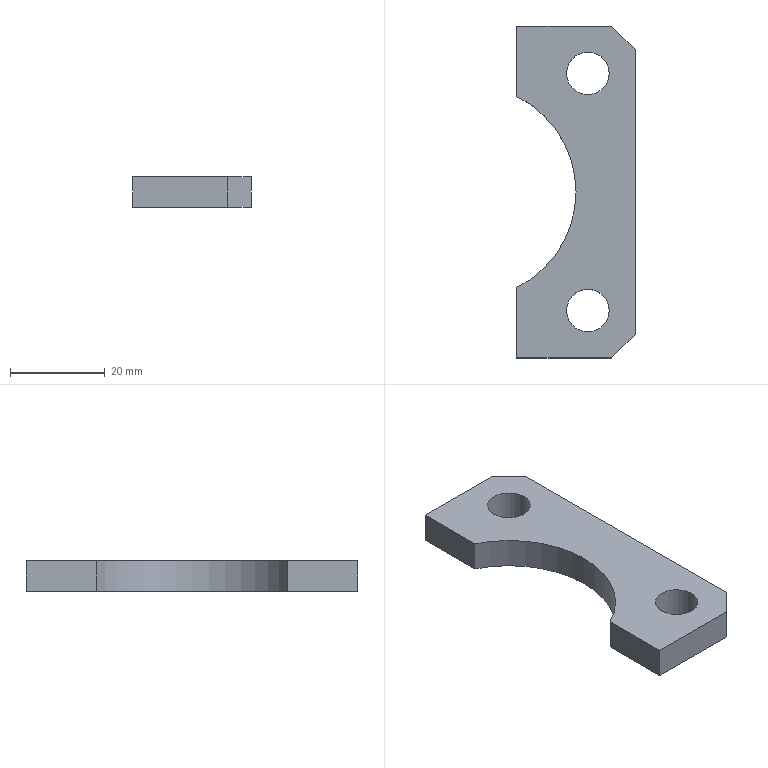Part | NX | features solid 2 | 1 solid | 12 faces | box 25 x 70 x 6.5 mm | volume 8042 mm3 | plane 9 | cylinder 3 | commonest cylinder face diameters 9 x2 45 x1
STEP:
#1=CARTESIAN_POINT('',(-840.,-430.,-48.49));
#2=VERTEX_POINT('',#1);
#3=CARTESIAN_POINT('',(-840.,-490.,-48.49));
#4=VERTEX_POINT('',#3);
#5=CARTESIAN_POINT('',(-840.,-325.,-48.49));
#6=DIRECTION('',(0.,1.,0.));
#7=VECTOR('',#6,1000.);
#8=LINE('',#5,#7);
#9=EDGE_CURVE('',#2,#4,#8,.F.);
#10=ORIENTED_EDGE('',*,*,#9,.T.);
#11=CARTESIAN_POINT('',(-840.,-490.,-54.99));
#12=VERTEX_POINT('',#11);
#13=CARTESIAN_POINT('',(-840.,-490.,-54.99));
#14=DIRECTION('',(0.,0.,-1.));
#15=VECTOR('',#14,1000.);
#16=LINE('',#13,#15);
#17=EDGE_CURVE('',#4,#12,#16,.T.);
#18=ORIENTED_EDGE('',*,*,#17,.T.);
#19=CARTESIAN_POINT('',(-840.,-430.,-54.99));
#20=VERTEX_POINT('',#19);
#21=CARTESIAN_POINT('',(-840.,-325.,-54.99));
#22=DIRECTION('',(0.,1.,0.));
#23=VECTOR('',#22,1000.);
#24=LINE('',#21,#23);
#25=EDGE_CURVE('',#20,#12,#24,.F.);
#26=ORIENTED_EDGE('',*,*,#25,.F.);
#27=CARTESIAN_POINT('',(-840.,-430.,-48.49));
#28=DIRECTION('',(0.,0.,1.));
#29=VECTOR('',#28,1000.);
#30=LINE('',#27,#29);
#31=EDGE_CURVE('',#20,#2,#30,.T.);
#32=ORIENTED_EDGE('',*,*,#31,.T.);
#33=EDGE_LOOP('',(#10,#18,#26,#32));
#34=FACE_BOUND('',#33,.T.);
#35=CARTESIAN_POINT('',(-840.,-325.,-54.99));
#36=DIRECTION('',(-1.,0.,0.));
#37=DIRECTION('',(0.,0.,-1.));
#38=AXIS2_PLACEMENT_3D('',#35,#36,#37);
#39=PLANE('',#38);
#40=ADVANCED_FACE('',(#34),#39,.F.);
#41=CARTESIAN_POINT('',(-865.,-439.844,-48.49));
#42=VERTEX_POINT('',#41);
#43=CARTESIAN_POINT('',(-865.,-439.844,-54.99));
#44=VERTEX_POINT('',#43);
#45=CARTESIAN_POINT('',(-865.,-439.844,-54.99));
#46=DIRECTION('',(0.,0.,1.));
#47=VECTOR('',#46,1000.);
#48=LINE('',#45,#47);
#49=EDGE_CURVE('',#42,#44,#48,.F.);
#50=ORIENTED_EDGE('',*,*,#49,.T.);
#51=CARTESIAN_POINT('',(-865.,-480.156,-54.99));
#52=VERTEX_POINT('',#51);
#53=CARTESIAN_POINT('',(-875.,-460.,-54.99));
#54=DIRECTION('',(0.,0.,1.));
#55=DIRECTION('',(-1.,0.,0.));
#56=AXIS2_PLACEMENT_3D('',#53,#54,#55);
#57=CIRCLE('',#56,22.5);
#58=EDGE_CURVE('',#52,#44,#57,.T.);
#59=ORIENTED_EDGE('',*,*,#58,.F.);
#60=CARTESIAN_POINT('',(-865.,-480.156,-48.49));
#61=VERTEX_POINT('',#60);
#62=CARTESIAN_POINT('',(-865.,-480.156,-54.99));
#63=DIRECTION('',(0.,0.,1.));
#64=VECTOR('',#63,1000.);
#65=LINE('',#62,#64);
#66=EDGE_CURVE('',#52,#61,#65,.T.);
#67=ORIENTED_EDGE('',*,*,#66,.T.);
#68=CARTESIAN_POINT('',(-875.,-460.,-48.49));
#69=DIRECTION('',(0.,0.,1.));
#70=DIRECTION('',(-1.,0.,0.));
#71=AXIS2_PLACEMENT_3D('',#68,#69,#70);
#72=CIRCLE('',#71,22.5);
#73=EDGE_CURVE('',#42,#61,#72,.F.);
#74=ORIENTED_EDGE('',*,*,#73,.F.);
#75=EDGE_LOOP('',(#50,#59,#67,#74));
#76=FACE_BOUND('',#75,.T.);
#77=CARTESIAN_POINT('',(-875.,-460.,-54.99));
#78=DIRECTION('',(0.,0.,1.));
#79=DIRECTION('',(-1.,0.,0.));
#80=AXIS2_PLACEMENT_3D('',#77,#78,#79);
#81=CYLINDRICAL_SURFACE('',#80,22.5);
#82=ADVANCED_FACE('',(#76),#81,.F.);
#83=CARTESIAN_POINT('',(-845.5,-485.,-48.49));
#84=VERTEX_POINT('',#83);
#85=CARTESIAN_POINT('',(-850.,-485.,-48.49));
#86=DIRECTION('',(0.,0.,-1.));
#87=DIRECTION('',(1.,0.,0.));
#88=AXIS2_PLACEMENT_3D('',#85,#86,#87);
#89=CIRCLE('',#88,4.5);
#90=EDGE_CURVE('',#84,#84,#89,.T.);
#91=ORIENTED_EDGE('',*,*,#90,.T.);
#92=EDGE_LOOP('',(#91));
#93=FACE_BOUND('',#92,.T.);
#94=CARTESIAN_POINT('',(-845.5,-435.,-48.49));
#95=VERTEX_POINT('',#94);
#96=CARTESIAN_POINT('',(-850.,-435.,-48.49));
#97=DIRECTION('',(0.,0.,-1.));
#98=DIRECTION('',(1.,0.,0.));
#99=AXIS2_PLACEMENT_3D('',#96,#97,#98);
#100=CIRCLE('',#99,4.5);
#101=EDGE_CURVE('',#95,#95,#100,.T.);
#102=ORIENTED_EDGE('',*,*,#101,.T.);
#103=EDGE_LOOP('',(#102));
#104=FACE_BOUND('',#103,.T.);
#105=CARTESIAN_POINT('',(-845.,-495.,-48.49));
#106=VERTEX_POINT('',#105);
#107=CARTESIAN_POINT('',(-865.,-495.,-48.49));
#108=VERTEX_POINT('',#107);
#109=CARTESIAN_POINT('',(-1090.,-495.,-48.49));
#110=DIRECTION('',(1.,0.,0.));
#111=VECTOR('',#110,1000.);
#112=LINE('',#109,#111);
#113=EDGE_CURVE('',#106,#108,#112,.F.);
#114=ORIENTED_EDGE('',*,*,#113,.F.);
#115=CARTESIAN_POINT('',(-845.,-495.,-48.49));
#116=DIRECTION('',(0.7071,0.7071,0.));
#117=VECTOR('',#116,1000.);
#118=LINE('',#115,#117);
#119=EDGE_CURVE('',#106,#4,#118,.T.);
#120=ORIENTED_EDGE('',*,*,#119,.T.);
#121=ORIENTED_EDGE('',*,*,#9,.F.);
#122=CARTESIAN_POINT('',(-845.,-425.,-48.49));
#123=VERTEX_POINT('',#122);
#124=CARTESIAN_POINT('',(-840.,-430.,-48.49));
#125=DIRECTION('',(0.7071,-0.7071,0.));
#126=VECTOR('',#125,1000.);
#127=LINE('',#124,#126);
#128=EDGE_CURVE('',#2,#123,#127,.F.);
#129=ORIENTED_EDGE('',*,*,#128,.T.);
#130=CARTESIAN_POINT('',(-865.,-425.,-48.49));
#131=VERTEX_POINT('',#130);
#132=CARTESIAN_POINT('',(-1090.,-425.,-48.49));
#133=DIRECTION('',(1.,0.,0.));
#134=VECTOR('',#133,1000.);
#135=LINE('',#132,#134);
#136=EDGE_CURVE('',#123,#131,#135,.F.);
#137=ORIENTED_EDGE('',*,*,#136,.T.);
#138=CARTESIAN_POINT('',(-865.,-325.,-48.49));
#139=DIRECTION('',(0.,1.,0.));
#140=VECTOR('',#139,1000.);
#141=LINE('',#138,#140);
#142=EDGE_CURVE('',#131,#42,#141,.F.);
#143=ORIENTED_EDGE('',*,*,#142,.T.);
#144=ORIENTED_EDGE('',*,*,#73,.T.);
#145=CARTESIAN_POINT('',(-865.,-325.,-48.49));
#146=DIRECTION('',(0.,1.,0.));
#147=VECTOR('',#146,1000.);
#148=LINE('',#145,#147);
#149=EDGE_CURVE('',#61,#108,#148,.F.);
#150=ORIENTED_EDGE('',*,*,#149,.T.);
#151=EDGE_LOOP('',(#114,#120,#121,#129,#137,#143,#144,#150));
#152=FACE_BOUND('',#151,.T.);
#153=CARTESIAN_POINT('',(-1090.,-325.,-48.49));
#154=DIRECTION('',(0.,0.,1.));
#155=DIRECTION('',(1.,0.,0.));
#156=AXIS2_PLACEMENT_3D('',#153,#154,#155);
#157=PLANE('',#156);
#158=ADVANCED_FACE('',(#93,#104,#152),#157,.T.);
#159=CARTESIAN_POINT('',(-854.5,-485.,-54.99));
#160=VERTEX_POINT('',#159);
#161=CARTESIAN_POINT('',(-850.,-485.,-54.99));
#162=DIRECTION('',(0.,0.,1.));
#163=DIRECTION('',(-1.,0.,0.));
#164=AXIS2_PLACEMENT_3D('',#161,#162,#163);
#165=CIRCLE('',#164,4.5);
#166=EDGE_CURVE('',#160,#160,#165,.F.);
#167=ORIENTED_EDGE('',*,*,#166,.F.);
#168=EDGE_LOOP('',(#167));
#169=FACE_BOUND('',#168,.T.);
#170=CARTESIAN_POINT('',(-854.5,-435.,-54.99));
#171=VERTEX_POINT('',#170);
#172=CARTESIAN_POINT('',(-850.,-435.,-54.99));
#173=DIRECTION('',(0.,0.,1.));
#174=DIRECTION('',(-1.,0.,0.));
#175=AXIS2_PLACEMENT_3D('',#172,#173,#174);
#176=CIRCLE('',#175,4.5);
#177=EDGE_CURVE('',#171,#171,#176,.F.);
#178=ORIENTED_EDGE('',*,*,#177,.F.);
#179=EDGE_LOOP('',(#178));
#180=FACE_BOUND('',#179,.T.);
#181=ORIENTED_EDGE('',*,*,#25,.T.);
#182=CARTESIAN_POINT('',(-845.,-495.,-54.99));
#183=VERTEX_POINT('',#182);
#184=CARTESIAN_POINT('',(-882.5,-532.5,-54.99));
#185=DIRECTION('',(-0.7071,-0.7071,0.));
#186=VECTOR('',#185,1000.);
#187=LINE('',#184,#186);
#188=EDGE_CURVE('',#12,#183,#187,.T.);
#189=ORIENTED_EDGE('',*,*,#188,.T.);
#190=CARTESIAN_POINT('',(-865.,-495.,-54.99));
#191=VERTEX_POINT('',#190);
#192=CARTESIAN_POINT('',(-1090.,-495.,-54.99));
#193=DIRECTION('',(1.,0.,0.));
#194=VECTOR('',#193,1000.);
#195=LINE('',#192,#194);
#196=EDGE_CURVE('',#183,#191,#195,.F.);
#197=ORIENTED_EDGE('',*,*,#196,.T.);
#198=CARTESIAN_POINT('',(-865.,-325.,-54.99));
#199=DIRECTION('',(0.,1.,0.));
#200=VECTOR('',#199,1000.);
#201=LINE('',#198,#200);
#202=EDGE_CURVE('',#52,#191,#201,.F.);
#203=ORIENTED_EDGE('',*,*,#202,.F.);
#204=ORIENTED_EDGE('',*,*,#58,.T.);
#205=CARTESIAN_POINT('',(-865.,-425.,-54.99));
#206=VERTEX_POINT('',#205);
#207=CARTESIAN_POINT('',(-865.,-325.,-54.99));
#208=DIRECTION('',(0.,1.,0.));
#209=VECTOR('',#208,1000.);
#210=LINE('',#207,#209);
#211=EDGE_CURVE('',#206,#44,#210,.F.);
#212=ORIENTED_EDGE('',*,*,#211,.F.);
#213=CARTESIAN_POINT('',(-845.,-425.,-54.99));
#214=VERTEX_POINT('',#213);
#215=CARTESIAN_POINT('',(-1090.,-425.,-54.99));
#216=DIRECTION('',(1.,0.,0.));
#217=VECTOR('',#216,1000.);
#218=LINE('',#215,#217);
#219=EDGE_CURVE('',#214,#206,#218,.F.);
#220=ORIENTED_EDGE('',*,*,#219,.F.);
#221=CARTESIAN_POINT('',(-1017.5,-252.5,-54.99));
#222=DIRECTION('',(-0.7071,0.7071,0.));
#223=VECTOR('',#222,1000.);
#224=LINE('',#221,#223);
#225=EDGE_CURVE('',#214,#20,#224,.F.);
#226=ORIENTED_EDGE('',*,*,#225,.T.);
#227=EDGE_LOOP('',(#181,#189,#197,#203,#204,#212,#220,#226));
#228=FACE_BOUND('',#227,.T.);
#229=CARTESIAN_POINT('',(-1090.,-325.,-54.99));
#230=DIRECTION('',(0.,0.,1.));
#231=DIRECTION('',(1.,0.,0.));
#232=AXIS2_PLACEMENT_3D('',#229,#230,#231);
#233=PLANE('',#232);
#234=ADVANCED_FACE('',(#169,#180,#228),#233,.F.);
#235=ORIENTED_EDGE('',*,*,#136,.F.);
#236=CARTESIAN_POINT('',(-845.,-425.,-54.99));
#237=DIRECTION('',(0.,0.,-1.));
#238=VECTOR('',#237,1000.);
#239=LINE('',#236,#238);
#240=EDGE_CURVE('',#123,#214,#239,.T.);
#241=ORIENTED_EDGE('',*,*,#240,.T.);
#242=ORIENTED_EDGE('',*,*,#219,.T.);
#243=CARTESIAN_POINT('',(-865.,-425.,-54.99));
#244=DIRECTION('',(0.,0.,-1.));
#245=VECTOR('',#244,1000.);
#246=LINE('',#243,#245);
#247=EDGE_CURVE('',#131,#206,#246,.T.);
#248=ORIENTED_EDGE('',*,*,#247,.F.);
#249=EDGE_LOOP('',(#235,#241,#242,#248));
#250=FACE_BOUND('',#249,.T.);
#251=CARTESIAN_POINT('',(-1090.,-425.,-54.99));
#252=DIRECTION('',(0.,1.,0.));
#253=DIRECTION('',(-1.,0.,0.));
#254=AXIS2_PLACEMENT_3D('',#251,#252,#253);
#255=PLANE('',#254);
#256=ADVANCED_FACE('',(#250),#255,.T.);
#257=ORIENTED_EDGE('',*,*,#196,.F.);
#258=CARTESIAN_POINT('',(-845.,-495.,-54.99));
#259=DIRECTION('',(0.,0.,1.));
#260=VECTOR('',#259,1000.);
#261=LINE('',#258,#260);
#262=EDGE_CURVE('',#183,#106,#261,.T.);
#263=ORIENTED_EDGE('',*,*,#262,.T.);
#264=ORIENTED_EDGE('',*,*,#113,.T.);
#265=CARTESIAN_POINT('',(-865.,-495.,-54.99));
#266=DIRECTION('',(0.,0.,-1.));
#267=VECTOR('',#266,1000.);
#268=LINE('',#265,#267);
#269=EDGE_CURVE('',#108,#191,#268,.T.);
#270=ORIENTED_EDGE('',*,*,#269,.T.);
#271=EDGE_LOOP('',(#257,#263,#264,#270));
#272=FACE_BOUND('',#271,.T.);
#273=CARTESIAN_POINT('',(-1090.,-495.,-54.99));
#274=DIRECTION('',(0.,1.,0.));
#275=DIRECTION('',(0.,0.,-1.));
#276=AXIS2_PLACEMENT_3D('',#273,#274,#275);
#277=PLANE('',#276);
#278=ADVANCED_FACE('',(#272),#277,.F.);
#279=ORIENTED_EDGE('',*,*,#149,.F.);
#280=ORIENTED_EDGE('',*,*,#66,.F.);
#281=ORIENTED_EDGE('',*,*,#202,.T.);
#282=ORIENTED_EDGE('',*,*,#269,.F.);
#283=EDGE_LOOP('',(#279,#280,#281,#282));
#284=FACE_BOUND('',#283,.T.);
#285=CARTESIAN_POINT('',(-865.,-425.,-54.99));
#286=DIRECTION('',(1.,0.,0.));
#287=DIRECTION('',(0.,0.,1.));
#288=AXIS2_PLACEMENT_3D('',#285,#286,#287);
#289=PLANE('',#288);
#290=ADVANCED_FACE('',(#284),#289,.F.);
#291=ORIENTED_EDGE('',*,*,#247,.T.);
#292=ORIENTED_EDGE('',*,*,#211,.T.);
#293=ORIENTED_EDGE('',*,*,#49,.F.);
#294=ORIENTED_EDGE('',*,*,#142,.F.);
#295=EDGE_LOOP('',(#291,#292,#293,#294));
#296=FACE_BOUND('',#295,.T.);
#297=CARTESIAN_POINT('',(-865.,-425.,-54.99));
#298=DIRECTION('',(1.,0.,0.));
#299=DIRECTION('',(0.,0.,1.));
#300=AXIS2_PLACEMENT_3D('',#297,#298,#299);
#301=PLANE('',#300);
#302=ADVANCED_FACE('',(#296),#301,.F.);
#303=ORIENTED_EDGE('',*,*,#177,.T.);
#304=EDGE_LOOP('',(#303));
#305=FACE_BOUND('',#304,.T.);
#306=ORIENTED_EDGE('',*,*,#101,.F.);
#307=EDGE_LOOP('',(#306));
#308=FACE_BOUND('',#307,.T.);
#309=CARTESIAN_POINT('',(-850.,-435.,-48.49));
#310=DIRECTION('',(0.,0.,-1.));
#311=DIRECTION('',(1.,0.,0.));
#312=AXIS2_PLACEMENT_3D('',#309,#310,#311);
#313=CYLINDRICAL_SURFACE('',#312,4.5);
#314=ADVANCED_FACE('',(#305,#308),#313,.F.);
#315=ORIENTED_EDGE('',*,*,#166,.T.);
#316=EDGE_LOOP('',(#315));
#317=FACE_BOUND('',#316,.T.);
#318=ORIENTED_EDGE('',*,*,#90,.F.);
#319=EDGE_LOOP('',(#318));
#320=FACE_BOUND('',#319,.T.);
#321=CARTESIAN_POINT('',(-850.,-485.,-48.49));
#322=DIRECTION('',(0.,0.,-1.));
#323=DIRECTION('',(1.,0.,0.));
#324=AXIS2_PLACEMENT_3D('',#321,#322,#323);
#325=CYLINDRICAL_SURFACE('',#324,4.5);
#326=ADVANCED_FACE('',(#317,#320),#325,.F.);
#327=ORIENTED_EDGE('',*,*,#188,.F.);
#328=ORIENTED_EDGE('',*,*,#17,.F.);
#329=ORIENTED_EDGE('',*,*,#119,.F.);
#330=ORIENTED_EDGE('',*,*,#262,.F.);
#331=EDGE_LOOP('',(#327,#328,#329,#330));
#332=FACE_BOUND('',#331,.T.);
#333=CARTESIAN_POINT('',(-845.,-495.,-54.99));
#334=DIRECTION('',(-0.7071,0.7071,0.));
#335=DIRECTION('',(-0.7071,-0.7071,0.));
#336=AXIS2_PLACEMENT_3D('',#333,#334,#335);
#337=PLANE('',#336);
#338=ADVANCED_FACE('',(#332),#337,.F.);
#339=ORIENTED_EDGE('',*,*,#225,.F.);
#340=ORIENTED_EDGE('',*,*,#240,.F.);
#341=ORIENTED_EDGE('',*,*,#128,.F.);
#342=ORIENTED_EDGE('',*,*,#31,.F.);
#343=EDGE_LOOP('',(#339,#340,#341,#342));
#344=FACE_BOUND('',#343,.T.);
#345=CARTESIAN_POINT('',(-840.,-430.,-54.99));
#346=DIRECTION('',(0.7071,0.7071,0.));
#347=DIRECTION('',(-0.7071,0.7071,0.));
#348=AXIS2_PLACEMENT_3D('',#345,#346,#347);
#349=PLANE('',#348);
#350=ADVANCED_FACE('',(#344),#349,.T.);
#351=CLOSED_SHELL('',(#40,#82,#158,#234,#256,#278,#290,#302,#314,#326,#338,#350));
#352=MANIFOLD_SOLID_BREP('',#351);
#353=(LENGTH_UNIT()NAMED_UNIT(*)SI_UNIT(.MILLI.,.METRE.));
#354=UNCERTAINTY_MEASURE_WITH_UNIT(LENGTH_MEASURE(0.00001),#353,'','');
#355=(NAMED_UNIT(*)PLANE_ANGLE_UNIT()SI_UNIT($,.RADIAN.));
#356=(NAMED_UNIT(*)SI_UNIT($,.STERADIAN.)SOLID_ANGLE_UNIT());
#357=(GEOMETRIC_REPRESENTATION_CONTEXT(3)GLOBAL_UNCERTAINTY_ASSIGNED_CONTEXT((#354))GLOBAL_UNIT_ASSIGNED_CONTEXT((#353,#355,#356))REPRESENTATION_CONTEXT('',''));
#358=ADVANCED_BREP_SHAPE_REPRESENTATION('',(#352),#357);